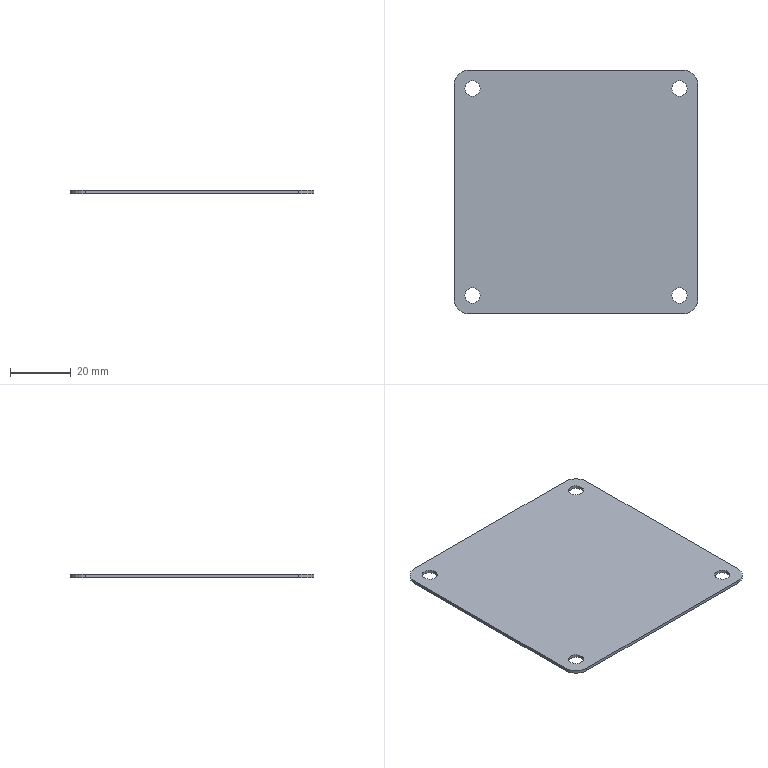Part | SolidWorks | features BaseBody 1 | 1 solid | 18 faces | box 80 x 80 x 1 mm | volume 6300 mm3 | cylinder 12 | plane 6 | commonest cylinder face diameters 5 x8 10 x4
STEP:
#1=CARTESIAN_POINT('',(-36.441,-33.941,1.));
#2=VERTEX_POINT('',#1);
#3=CARTESIAN_POINT('',(-31.441,-33.941,1.));
#4=VERTEX_POINT('',#3);
#5=CARTESIAN_POINT('',(-33.941,-33.941,1.));
#6=DIRECTION('',(0.,0.,1.));
#7=DIRECTION('',(-1.,0.,0.));
#8=AXIS2_PLACEMENT_3D('',#5,#6,#7);
#9=CIRCLE('',#8,2.5);
#10=EDGE_CURVE('',#2,#4,#9,.T.);
#11=ORIENTED_EDGE('',*,*,#10,.T.);
#12=CARTESIAN_POINT('',(-31.441,-33.941,0.));
#13=VERTEX_POINT('',#12);
#14=CARTESIAN_POINT('',(-31.441,-33.941,1.));
#15=DIRECTION('',(0.,0.,-1.));
#16=VECTOR('',#15,1000.);
#17=LINE('',#14,#16);
#18=EDGE_CURVE('',#4,#13,#17,.T.);
#19=ORIENTED_EDGE('',*,*,#18,.T.);
#20=CARTESIAN_POINT('',(-36.441,-33.941,0.));
#21=VERTEX_POINT('',#20);
#22=CARTESIAN_POINT('',(-33.941,-33.941,0.));
#23=DIRECTION('',(0.,0.,1.));
#24=DIRECTION('',(-1.,0.,0.));
#25=AXIS2_PLACEMENT_3D('',#22,#23,#24);
#26=CIRCLE('',#25,2.5);
#27=EDGE_CURVE('',#21,#13,#26,.T.);
#28=ORIENTED_EDGE('',*,*,#27,.F.);
#29=CARTESIAN_POINT('',(-36.441,-33.941,1.));
#30=DIRECTION('',(0.,0.,-1.));
#31=VECTOR('',#30,1000.);
#32=LINE('',#29,#31);
#33=EDGE_CURVE('',#2,#21,#32,.T.);
#34=ORIENTED_EDGE('',*,*,#33,.F.);
#35=EDGE_LOOP('',(#11,#19,#28,#34));
#36=FACE_OUTER_BOUND('',#35,.T.);
#37=CARTESIAN_POINT('',(-33.941,-33.941,1.));
#38=DIRECTION('',(0.,0.,-1.));
#39=DIRECTION('',(-1.,0.,0.));
#40=AXIS2_PLACEMENT_3D('',#37,#38,#39);
#41=CYLINDRICAL_SURFACE('',#40,2.5);
#42=ADVANCED_FACE('',(#36),#41,.F.);
#43=CARTESIAN_POINT('',(31.441,-33.941,1.));
#44=VERTEX_POINT('',#43);
#45=CARTESIAN_POINT('',(36.441,-33.941,1.));
#46=VERTEX_POINT('',#45);
#47=CARTESIAN_POINT('',(33.941,-33.941,1.));
#48=DIRECTION('',(0.,0.,1.));
#49=DIRECTION('',(-1.,0.,0.));
#50=AXIS2_PLACEMENT_3D('',#47,#48,#49);
#51=CIRCLE('',#50,2.5);
#52=EDGE_CURVE('',#44,#46,#51,.T.);
#53=ORIENTED_EDGE('',*,*,#52,.T.);
#54=CARTESIAN_POINT('',(36.441,-33.941,0.));
#55=VERTEX_POINT('',#54);
#56=CARTESIAN_POINT('',(36.441,-33.941,1.));
#57=DIRECTION('',(0.,0.,-1.));
#58=VECTOR('',#57,1000.);
#59=LINE('',#56,#58);
#60=EDGE_CURVE('',#46,#55,#59,.T.);
#61=ORIENTED_EDGE('',*,*,#60,.T.);
#62=CARTESIAN_POINT('',(31.441,-33.941,0.));
#63=VERTEX_POINT('',#62);
#64=CARTESIAN_POINT('',(33.941,-33.941,0.));
#65=DIRECTION('',(0.,0.,1.));
#66=DIRECTION('',(-1.,0.,0.));
#67=AXIS2_PLACEMENT_3D('',#64,#65,#66);
#68=CIRCLE('',#67,2.5);
#69=EDGE_CURVE('',#63,#55,#68,.T.);
#70=ORIENTED_EDGE('',*,*,#69,.F.);
#71=CARTESIAN_POINT('',(31.441,-33.941,1.));
#72=DIRECTION('',(0.,0.,-1.));
#73=VECTOR('',#72,1000.);
#74=LINE('',#71,#73);
#75=EDGE_CURVE('',#44,#63,#74,.T.);
#76=ORIENTED_EDGE('',*,*,#75,.F.);
#77=EDGE_LOOP('',(#53,#61,#70,#76));
#78=FACE_OUTER_BOUND('',#77,.T.);
#79=CARTESIAN_POINT('',(33.941,-33.941,1.));
#80=DIRECTION('',(0.,0.,-1.));
#81=DIRECTION('',(-1.,0.,0.));
#82=AXIS2_PLACEMENT_3D('',#79,#80,#81);
#83=CYLINDRICAL_SURFACE('',#82,2.5);
#84=ADVANCED_FACE('',(#78),#83,.F.);
#85=CARTESIAN_POINT('',(31.441,33.941,1.));
#86=VERTEX_POINT('',#85);
#87=CARTESIAN_POINT('',(36.441,33.941,1.));
#88=VERTEX_POINT('',#87);
#89=CARTESIAN_POINT('',(33.941,33.941,1.));
#90=DIRECTION('',(0.,0.,1.));
#91=DIRECTION('',(-1.,0.,0.));
#92=AXIS2_PLACEMENT_3D('',#89,#90,#91);
#93=CIRCLE('',#92,2.5);
#94=EDGE_CURVE('',#86,#88,#93,.T.);
#95=ORIENTED_EDGE('',*,*,#94,.T.);
#96=CARTESIAN_POINT('',(36.441,33.941,0.));
#97=VERTEX_POINT('',#96);
#98=CARTESIAN_POINT('',(36.441,33.941,1.));
#99=DIRECTION('',(0.,0.,-1.));
#100=VECTOR('',#99,1000.);
#101=LINE('',#98,#100);
#102=EDGE_CURVE('',#88,#97,#101,.T.);
#103=ORIENTED_EDGE('',*,*,#102,.T.);
#104=CARTESIAN_POINT('',(31.441,33.941,0.));
#105=VERTEX_POINT('',#104);
#106=CARTESIAN_POINT('',(33.941,33.941,0.));
#107=DIRECTION('',(0.,0.,1.));
#108=DIRECTION('',(-1.,0.,0.));
#109=AXIS2_PLACEMENT_3D('',#106,#107,#108);
#110=CIRCLE('',#109,2.5);
#111=EDGE_CURVE('',#105,#97,#110,.T.);
#112=ORIENTED_EDGE('',*,*,#111,.F.);
#113=CARTESIAN_POINT('',(31.441,33.941,1.));
#114=DIRECTION('',(0.,0.,-1.));
#115=VECTOR('',#114,1000.);
#116=LINE('',#113,#115);
#117=EDGE_CURVE('',#86,#105,#116,.T.);
#118=ORIENTED_EDGE('',*,*,#117,.F.);
#119=EDGE_LOOP('',(#95,#103,#112,#118));
#120=FACE_OUTER_BOUND('',#119,.T.);
#121=CARTESIAN_POINT('',(33.941,33.941,1.));
#122=DIRECTION('',(0.,0.,-1.));
#123=DIRECTION('',(-1.,0.,0.));
#124=AXIS2_PLACEMENT_3D('',#121,#122,#123);
#125=CYLINDRICAL_SURFACE('',#124,2.5);
#126=ADVANCED_FACE('',(#120),#125,.F.);
#127=CARTESIAN_POINT('',(-36.441,33.941,1.));
#128=VERTEX_POINT('',#127);
#129=CARTESIAN_POINT('',(-31.441,33.941,1.));
#130=VERTEX_POINT('',#129);
#131=CARTESIAN_POINT('',(-33.941,33.941,1.));
#132=DIRECTION('',(0.,0.,1.));
#133=DIRECTION('',(-1.,0.,0.));
#134=AXIS2_PLACEMENT_3D('',#131,#132,#133);
#135=CIRCLE('',#134,2.5);
#136=EDGE_CURVE('',#128,#130,#135,.T.);
#137=ORIENTED_EDGE('',*,*,#136,.T.);
#138=CARTESIAN_POINT('',(-31.441,33.941,0.));
#139=VERTEX_POINT('',#138);
#140=CARTESIAN_POINT('',(-31.441,33.941,1.));
#141=DIRECTION('',(0.,0.,-1.));
#142=VECTOR('',#141,1000.);
#143=LINE('',#140,#142);
#144=EDGE_CURVE('',#130,#139,#143,.T.);
#145=ORIENTED_EDGE('',*,*,#144,.T.);
#146=CARTESIAN_POINT('',(-36.441,33.941,0.));
#147=VERTEX_POINT('',#146);
#148=CARTESIAN_POINT('',(-33.941,33.941,0.));
#149=DIRECTION('',(0.,0.,1.));
#150=DIRECTION('',(-1.,0.,0.));
#151=AXIS2_PLACEMENT_3D('',#148,#149,#150);
#152=CIRCLE('',#151,2.5);
#153=EDGE_CURVE('',#147,#139,#152,.T.);
#154=ORIENTED_EDGE('',*,*,#153,.F.);
#155=CARTESIAN_POINT('',(-36.441,33.941,1.));
#156=DIRECTION('',(0.,0.,-1.));
#157=VECTOR('',#156,1000.);
#158=LINE('',#155,#157);
#159=EDGE_CURVE('',#128,#147,#158,.T.);
#160=ORIENTED_EDGE('',*,*,#159,.F.);
#161=EDGE_LOOP('',(#137,#145,#154,#160));
#162=FACE_OUTER_BOUND('',#161,.T.);
#163=CARTESIAN_POINT('',(-33.941,33.941,1.));
#164=DIRECTION('',(0.,0.,-1.));
#165=DIRECTION('',(-1.,0.,0.));
#166=AXIS2_PLACEMENT_3D('',#163,#164,#165);
#167=CYLINDRICAL_SURFACE('',#166,2.5);
#168=ADVANCED_FACE('',(#162),#167,.F.);
#169=ORIENTED_EDGE('',*,*,#10,.F.);
#170=CARTESIAN_POINT('',(-33.941,-33.941,1.));
#171=DIRECTION('',(0.,0.,1.));
#172=DIRECTION('',(-1.,0.,0.));
#173=AXIS2_PLACEMENT_3D('',#170,#171,#172);
#174=CIRCLE('',#173,2.5);
#175=EDGE_CURVE('',#4,#2,#174,.T.);
#176=ORIENTED_EDGE('',*,*,#175,.F.);
#177=EDGE_LOOP('',(#169,#176));
#178=FACE_BOUND('',#177,.T.);
#179=ORIENTED_EDGE('',*,*,#52,.F.);
#180=CARTESIAN_POINT('',(33.941,-33.941,1.));
#181=DIRECTION('',(0.,0.,1.));
#182=DIRECTION('',(-1.,0.,0.));
#183=AXIS2_PLACEMENT_3D('',#180,#181,#182);
#184=CIRCLE('',#183,2.5);
#185=EDGE_CURVE('',#46,#44,#184,.T.);
#186=ORIENTED_EDGE('',*,*,#185,.F.);
#187=EDGE_LOOP('',(#179,#186));
#188=FACE_BOUND('',#187,.T.);
#189=ORIENTED_EDGE('',*,*,#94,.F.);
#190=CARTESIAN_POINT('',(33.941,33.941,1.));
#191=DIRECTION('',(0.,0.,1.));
#192=DIRECTION('',(-1.,0.,0.));
#193=AXIS2_PLACEMENT_3D('',#190,#191,#192);
#194=CIRCLE('',#193,2.5);
#195=EDGE_CURVE('',#88,#86,#194,.T.);
#196=ORIENTED_EDGE('',*,*,#195,.F.);
#197=EDGE_LOOP('',(#189,#196));
#198=FACE_BOUND('',#197,.T.);
#199=ORIENTED_EDGE('',*,*,#136,.F.);
#200=CARTESIAN_POINT('',(-33.941,33.941,1.));
#201=DIRECTION('',(0.,0.,1.));
#202=DIRECTION('',(-1.,0.,0.));
#203=AXIS2_PLACEMENT_3D('',#200,#201,#202);
#204=CIRCLE('',#203,2.5);
#205=EDGE_CURVE('',#130,#128,#204,.T.);
#206=ORIENTED_EDGE('',*,*,#205,.F.);
#207=EDGE_LOOP('',(#199,#206));
#208=FACE_BOUND('',#207,.T.);
#209=CARTESIAN_POINT('',(35.,-40.,1.));
#210=VERTEX_POINT('',#209);
#211=CARTESIAN_POINT('',(-35.,-40.,1.));
#212=VERTEX_POINT('',#211);
#213=CARTESIAN_POINT('',(-35.,-40.,1.));
#214=DIRECTION('',(-1.,0.,0.));
#215=VECTOR('',#214,1000.);
#216=LINE('',#213,#215);
#217=EDGE_CURVE('',#210,#212,#216,.T.);
#218=ORIENTED_EDGE('',*,*,#217,.F.);
#219=CARTESIAN_POINT('',(40.,-35.,1.));
#220=VERTEX_POINT('',#219);
#221=CARTESIAN_POINT('',(35.,-35.,1.));
#222=DIRECTION('',(0.,0.,-1.));
#223=DIRECTION('',(-1.,0.,0.));
#224=AXIS2_PLACEMENT_3D('',#221,#222,#223);
#225=CIRCLE('',#224,5.);
#226=EDGE_CURVE('',#220,#210,#225,.T.);
#227=ORIENTED_EDGE('',*,*,#226,.F.);
#228=CARTESIAN_POINT('',(40.,35.,1.));
#229=VERTEX_POINT('',#228);
#230=CARTESIAN_POINT('',(40.,-35.,1.));
#231=DIRECTION('',(0.,-1.,0.));
#232=VECTOR('',#231,1000.);
#233=LINE('',#230,#232);
#234=EDGE_CURVE('',#229,#220,#233,.T.);
#235=ORIENTED_EDGE('',*,*,#234,.F.);
#236=CARTESIAN_POINT('',(35.,40.,1.));
#237=VERTEX_POINT('',#236);
#238=CARTESIAN_POINT('',(35.,35.,1.));
#239=DIRECTION('',(0.,0.,-1.));
#240=DIRECTION('',(-1.,0.,0.));
#241=AXIS2_PLACEMENT_3D('',#238,#239,#240);
#242=CIRCLE('',#241,5.);
#243=EDGE_CURVE('',#237,#229,#242,.T.);
#244=ORIENTED_EDGE('',*,*,#243,.F.);
#245=CARTESIAN_POINT('',(-35.,40.,1.));
#246=VERTEX_POINT('',#245);
#247=CARTESIAN_POINT('',(-35.,40.,1.));
#248=DIRECTION('',(1.,0.,0.));
#249=VECTOR('',#248,1000.);
#250=LINE('',#247,#249);
#251=EDGE_CURVE('',#246,#237,#250,.T.);
#252=ORIENTED_EDGE('',*,*,#251,.F.);
#253=CARTESIAN_POINT('',(-40.,35.,1.));
#254=VERTEX_POINT('',#253);
#255=CARTESIAN_POINT('',(-35.,35.,1.));
#256=DIRECTION('',(0.,0.,-1.));
#257=DIRECTION('',(-1.,0.,0.));
#258=AXIS2_PLACEMENT_3D('',#255,#256,#257);
#259=CIRCLE('',#258,5.);
#260=EDGE_CURVE('',#254,#246,#259,.T.);
#261=ORIENTED_EDGE('',*,*,#260,.F.);
#262=CARTESIAN_POINT('',(-40.,-35.,1.));
#263=VERTEX_POINT('',#262);
#264=CARTESIAN_POINT('',(-40.,-35.,1.));
#265=DIRECTION('',(0.,1.,0.));
#266=VECTOR('',#265,1000.);
#267=LINE('',#264,#266);
#268=EDGE_CURVE('',#263,#254,#267,.T.);
#269=ORIENTED_EDGE('',*,*,#268,.F.);
#270=CARTESIAN_POINT('',(-35.,-35.,1.));
#271=DIRECTION('',(0.,0.,-1.));
#272=DIRECTION('',(-1.,0.,0.));
#273=AXIS2_PLACEMENT_3D('',#270,#271,#272);
#274=CIRCLE('',#273,5.);
#275=EDGE_CURVE('',#212,#263,#274,.T.);
#276=ORIENTED_EDGE('',*,*,#275,.F.);
#277=EDGE_LOOP('',(#218,#227,#235,#244,#252,#261,#269,#276));
#278=FACE_OUTER_BOUND('',#277,.T.);
#279=CARTESIAN_POINT('',(-35.,-35.,1.));
#280=DIRECTION('',(0.,0.,-1.));
#281=DIRECTION('',(-1.,0.,0.));
#282=AXIS2_PLACEMENT_3D('',#279,#280,#281);
#283=PLANE('',#282);
#284=ADVANCED_FACE('',(#178,#188,#198,#208,#278),#283,.F.);
#285=ORIENTED_EDGE('',*,*,#18,.F.);
#286=ORIENTED_EDGE('',*,*,#175,.T.);
#287=ORIENTED_EDGE('',*,*,#33,.T.);
#288=CARTESIAN_POINT('',(-33.941,-33.941,0.));
#289=DIRECTION('',(0.,0.,1.));
#290=DIRECTION('',(-1.,0.,0.));
#291=AXIS2_PLACEMENT_3D('',#288,#289,#290);
#292=CIRCLE('',#291,2.5);
#293=EDGE_CURVE('',#13,#21,#292,.T.);
#294=ORIENTED_EDGE('',*,*,#293,.F.);
#295=EDGE_LOOP('',(#285,#286,#287,#294));
#296=FACE_OUTER_BOUND('',#295,.T.);
#297=CARTESIAN_POINT('',(-33.941,-33.941,1.));
#298=DIRECTION('',(0.,0.,-1.));
#299=DIRECTION('',(-1.,0.,0.));
#300=AXIS2_PLACEMENT_3D('',#297,#298,#299);
#301=CYLINDRICAL_SURFACE('',#300,2.5);
#302=ADVANCED_FACE('',(#296),#301,.F.);
#303=ORIENTED_EDGE('',*,*,#60,.F.);
#304=ORIENTED_EDGE('',*,*,#185,.T.);
#305=ORIENTED_EDGE('',*,*,#75,.T.);
#306=CARTESIAN_POINT('',(33.941,-33.941,0.));
#307=DIRECTION('',(0.,0.,1.));
#308=DIRECTION('',(-1.,0.,0.));
#309=AXIS2_PLACEMENT_3D('',#306,#307,#308);
#310=CIRCLE('',#309,2.5);
#311=EDGE_CURVE('',#55,#63,#310,.T.);
#312=ORIENTED_EDGE('',*,*,#311,.F.);
#313=EDGE_LOOP('',(#303,#304,#305,#312));
#314=FACE_OUTER_BOUND('',#313,.T.);
#315=CARTESIAN_POINT('',(33.941,-33.941,1.));
#316=DIRECTION('',(0.,0.,-1.));
#317=DIRECTION('',(-1.,0.,0.));
#318=AXIS2_PLACEMENT_3D('',#315,#316,#317);
#319=CYLINDRICAL_SURFACE('',#318,2.5);
#320=ADVANCED_FACE('',(#314),#319,.F.);
#321=ORIENTED_EDGE('',*,*,#102,.F.);
#322=ORIENTED_EDGE('',*,*,#195,.T.);
#323=ORIENTED_EDGE('',*,*,#117,.T.);
#324=CARTESIAN_POINT('',(33.941,33.941,0.));
#325=DIRECTION('',(0.,0.,1.));
#326=DIRECTION('',(-1.,0.,0.));
#327=AXIS2_PLACEMENT_3D('',#324,#325,#326);
#328=CIRCLE('',#327,2.5);
#329=EDGE_CURVE('',#97,#105,#328,.T.);
#330=ORIENTED_EDGE('',*,*,#329,.F.);
#331=EDGE_LOOP('',(#321,#322,#323,#330));
#332=FACE_OUTER_BOUND('',#331,.T.);
#333=CARTESIAN_POINT('',(33.941,33.941,1.));
#334=DIRECTION('',(0.,0.,-1.));
#335=DIRECTION('',(-1.,0.,0.));
#336=AXIS2_PLACEMENT_3D('',#333,#334,#335);
#337=CYLINDRICAL_SURFACE('',#336,2.5);
#338=ADVANCED_FACE('',(#332),#337,.F.);
#339=ORIENTED_EDGE('',*,*,#144,.F.);
#340=ORIENTED_EDGE('',*,*,#205,.T.);
#341=ORIENTED_EDGE('',*,*,#159,.T.);
#342=CARTESIAN_POINT('',(-33.941,33.941,0.));
#343=DIRECTION('',(0.,0.,1.));
#344=DIRECTION('',(-1.,0.,0.));
#345=AXIS2_PLACEMENT_3D('',#342,#343,#344);
#346=CIRCLE('',#345,2.5);
#347=EDGE_CURVE('',#139,#147,#346,.T.);
#348=ORIENTED_EDGE('',*,*,#347,.F.);
#349=EDGE_LOOP('',(#339,#340,#341,#348));
#350=FACE_OUTER_BOUND('',#349,.T.);
#351=CARTESIAN_POINT('',(-33.941,33.941,1.));
#352=DIRECTION('',(0.,0.,-1.));
#353=DIRECTION('',(-1.,0.,0.));
#354=AXIS2_PLACEMENT_3D('',#351,#352,#353);
#355=CYLINDRICAL_SURFACE('',#354,2.5);
#356=ADVANCED_FACE('',(#350),#355,.F.);
#357=ORIENTED_EDGE('',*,*,#275,.T.);
#358=CARTESIAN_POINT('',(-40.,-35.,0.));
#359=VERTEX_POINT('',#358);
#360=CARTESIAN_POINT('',(-40.,-35.,1.));
#361=DIRECTION('',(0.,0.,-1.));
#362=VECTOR('',#361,1000.);
#363=LINE('',#360,#362);
#364=EDGE_CURVE('',#263,#359,#363,.T.);
#365=ORIENTED_EDGE('',*,*,#364,.T.);
#366=CARTESIAN_POINT('',(-35.,-40.,0.));
#367=VERTEX_POINT('',#366);
#368=CARTESIAN_POINT('',(-35.,-35.,0.));
#369=DIRECTION('',(0.,0.,1.));
#370=DIRECTION('',(-1.,0.,0.));
#371=AXIS2_PLACEMENT_3D('',#368,#369,#370);
#372=CIRCLE('',#371,5.);
#373=EDGE_CURVE('',#359,#367,#372,.T.);
#374=ORIENTED_EDGE('',*,*,#373,.T.);
#375=CARTESIAN_POINT('',(-35.,-40.,1.));
#376=DIRECTION('',(0.,0.,1.));
#377=VECTOR('',#376,1000.);
#378=LINE('',#375,#377);
#379=EDGE_CURVE('',#367,#212,#378,.T.);
#380=ORIENTED_EDGE('',*,*,#379,.T.);
#381=EDGE_LOOP('',(#357,#365,#374,#380));
#382=FACE_OUTER_BOUND('',#381,.T.);
#383=CARTESIAN_POINT('',(-35.,-35.,1.));
#384=DIRECTION('',(0.,0.,-1.));
#385=DIRECTION('',(-1.,0.,0.));
#386=AXIS2_PLACEMENT_3D('',#383,#384,#385);
#387=CYLINDRICAL_SURFACE('',#386,5.);
#388=ADVANCED_FACE('',(#382),#387,.T.);
#389=CARTESIAN_POINT('',(35.,-40.,0.));
#390=VERTEX_POINT('',#389);
#391=CARTESIAN_POINT('',(35.,-40.,1.));
#392=DIRECTION('',(0.,0.,-1.));
#393=VECTOR('',#392,1000.);
#394=LINE('',#391,#393);
#395=EDGE_CURVE('',#210,#390,#394,.T.);
#396=ORIENTED_EDGE('',*,*,#395,.F.);
#397=ORIENTED_EDGE('',*,*,#217,.T.);
#398=ORIENTED_EDGE('',*,*,#379,.F.);
#399=CARTESIAN_POINT('',(35.,-40.,0.));
#400=DIRECTION('',(-1.,0.,0.));
#401=VECTOR('',#400,1000.);
#402=LINE('',#399,#401);
#403=EDGE_CURVE('',#390,#367,#402,.T.);
#404=ORIENTED_EDGE('',*,*,#403,.F.);
#405=EDGE_LOOP('',(#396,#397,#398,#404));
#406=FACE_OUTER_BOUND('',#405,.T.);
#407=CARTESIAN_POINT('',(35.,-40.,1.));
#408=DIRECTION('',(0.,1.,0.));
#409=DIRECTION('',(-1.,0.,0.));
#410=AXIS2_PLACEMENT_3D('',#407,#408,#409);
#411=PLANE('',#410);
#412=ADVANCED_FACE('',(#406),#411,.F.);
#413=ORIENTED_EDGE('',*,*,#226,.T.);
#414=ORIENTED_EDGE('',*,*,#395,.T.);
#415=CARTESIAN_POINT('',(40.,-35.,0.));
#416=VERTEX_POINT('',#415);
#417=CARTESIAN_POINT('',(35.,-35.,0.));
#418=DIRECTION('',(0.,0.,1.));
#419=DIRECTION('',(-1.,0.,0.));
#420=AXIS2_PLACEMENT_3D('',#417,#418,#419);
#421=CIRCLE('',#420,5.);
#422=EDGE_CURVE('',#390,#416,#421,.T.);
#423=ORIENTED_EDGE('',*,*,#422,.T.);
#424=CARTESIAN_POINT('',(40.,-35.,1.));
#425=DIRECTION('',(0.,0.,1.));
#426=VECTOR('',#425,1000.);
#427=LINE('',#424,#426);
#428=EDGE_CURVE('',#416,#220,#427,.T.);
#429=ORIENTED_EDGE('',*,*,#428,.T.);
#430=EDGE_LOOP('',(#413,#414,#423,#429));
#431=FACE_OUTER_BOUND('',#430,.T.);
#432=CARTESIAN_POINT('',(35.,-35.,1.));
#433=DIRECTION('',(0.,0.,-1.));
#434=DIRECTION('',(-1.,0.,0.));
#435=AXIS2_PLACEMENT_3D('',#432,#433,#434);
#436=CYLINDRICAL_SURFACE('',#435,5.);
#437=ADVANCED_FACE('',(#431),#436,.T.);
#438=CARTESIAN_POINT('',(40.,35.,0.));
#439=VERTEX_POINT('',#438);
#440=CARTESIAN_POINT('',(40.,35.,1.));
#441=DIRECTION('',(0.,0.,-1.));
#442=VECTOR('',#441,1000.);
#443=LINE('',#440,#442);
#444=EDGE_CURVE('',#229,#439,#443,.T.);
#445=ORIENTED_EDGE('',*,*,#444,.F.);
#446=ORIENTED_EDGE('',*,*,#234,.T.);
#447=ORIENTED_EDGE('',*,*,#428,.F.);
#448=CARTESIAN_POINT('',(40.,35.,0.));
#449=DIRECTION('',(0.,-1.,0.));
#450=VECTOR('',#449,1000.);
#451=LINE('',#448,#450);
#452=EDGE_CURVE('',#439,#416,#451,.T.);
#453=ORIENTED_EDGE('',*,*,#452,.F.);
#454=EDGE_LOOP('',(#445,#446,#447,#453));
#455=FACE_OUTER_BOUND('',#454,.T.);
#456=CARTESIAN_POINT('',(40.,35.,1.));
#457=DIRECTION('',(-1.,0.,0.));
#458=DIRECTION('',(0.,-1.,0.));
#459=AXIS2_PLACEMENT_3D('',#456,#457,#458);
#460=PLANE('',#459);
#461=ADVANCED_FACE('',(#455),#460,.F.);
#462=ORIENTED_EDGE('',*,*,#243,.T.);
#463=ORIENTED_EDGE('',*,*,#444,.T.);
#464=CARTESIAN_POINT('',(35.,40.,0.));
#465=VERTEX_POINT('',#464);
#466=CARTESIAN_POINT('',(35.,35.,0.));
#467=DIRECTION('',(0.,0.,1.));
#468=DIRECTION('',(-1.,0.,0.));
#469=AXIS2_PLACEMENT_3D('',#466,#467,#468);
#470=CIRCLE('',#469,5.);
#471=EDGE_CURVE('',#439,#465,#470,.T.);
#472=ORIENTED_EDGE('',*,*,#471,.T.);
#473=CARTESIAN_POINT('',(35.,40.,1.));
#474=DIRECTION('',(0.,0.,1.));
#475=VECTOR('',#474,1000.);
#476=LINE('',#473,#475);
#477=EDGE_CURVE('',#465,#237,#476,.T.);
#478=ORIENTED_EDGE('',*,*,#477,.T.);
#479=EDGE_LOOP('',(#462,#463,#472,#478));
#480=FACE_OUTER_BOUND('',#479,.T.);
#481=CARTESIAN_POINT('',(35.,35.,1.));
#482=DIRECTION('',(0.,0.,-1.));
#483=DIRECTION('',(-1.,0.,0.));
#484=AXIS2_PLACEMENT_3D('',#481,#482,#483);
#485=CYLINDRICAL_SURFACE('',#484,5.);
#486=ADVANCED_FACE('',(#480),#485,.T.);
#487=CARTESIAN_POINT('',(-35.,40.,0.));
#488=VERTEX_POINT('',#487);
#489=CARTESIAN_POINT('',(-35.,40.,1.));
#490=DIRECTION('',(0.,0.,-1.));
#491=VECTOR('',#490,1000.);
#492=LINE('',#489,#491);
#493=EDGE_CURVE('',#246,#488,#492,.T.);
#494=ORIENTED_EDGE('',*,*,#493,.F.);
#495=ORIENTED_EDGE('',*,*,#251,.T.);
#496=ORIENTED_EDGE('',*,*,#477,.F.);
#497=CARTESIAN_POINT('',(35.,40.,0.));
#498=DIRECTION('',(1.,0.,0.));
#499=VECTOR('',#498,1000.);
#500=LINE('',#497,#499);
#501=EDGE_CURVE('',#488,#465,#500,.T.);
#502=ORIENTED_EDGE('',*,*,#501,.F.);
#503=EDGE_LOOP('',(#494,#495,#496,#502));
#504=FACE_OUTER_BOUND('',#503,.T.);
#505=CARTESIAN_POINT('',(35.,40.,1.));
#506=DIRECTION('',(0.,-1.,0.));
#507=DIRECTION('',(1.,0.,0.));
#508=AXIS2_PLACEMENT_3D('',#505,#506,#507);
#509=PLANE('',#508);
#510=ADVANCED_FACE('',(#504),#509,.F.);
#511=ORIENTED_EDGE('',*,*,#260,.T.);
#512=ORIENTED_EDGE('',*,*,#493,.T.);
#513=CARTESIAN_POINT('',(-40.,35.,0.));
#514=VERTEX_POINT('',#513);
#515=CARTESIAN_POINT('',(-35.,35.,0.));
#516=DIRECTION('',(0.,0.,1.));
#517=DIRECTION('',(-1.,0.,0.));
#518=AXIS2_PLACEMENT_3D('',#515,#516,#517);
#519=CIRCLE('',#518,5.);
#520=EDGE_CURVE('',#488,#514,#519,.T.);
#521=ORIENTED_EDGE('',*,*,#520,.T.);
#522=CARTESIAN_POINT('',(-40.,35.,1.));
#523=DIRECTION('',(0.,0.,1.));
#524=VECTOR('',#523,1000.);
#525=LINE('',#522,#524);
#526=EDGE_CURVE('',#514,#254,#525,.T.);
#527=ORIENTED_EDGE('',*,*,#526,.T.);
#528=EDGE_LOOP('',(#511,#512,#521,#527));
#529=FACE_OUTER_BOUND('',#528,.T.);
#530=CARTESIAN_POINT('',(-35.,35.,1.));
#531=DIRECTION('',(0.,0.,-1.));
#532=DIRECTION('',(-1.,0.,0.));
#533=AXIS2_PLACEMENT_3D('',#530,#531,#532);
#534=CYLINDRICAL_SURFACE('',#533,5.);
#535=ADVANCED_FACE('',(#529),#534,.T.);
#536=ORIENTED_EDGE('',*,*,#364,.F.);
#537=ORIENTED_EDGE('',*,*,#268,.T.);
#538=ORIENTED_EDGE('',*,*,#526,.F.);
#539=CARTESIAN_POINT('',(-40.,35.,0.));
#540=DIRECTION('',(0.,1.,0.));
#541=VECTOR('',#540,1000.);
#542=LINE('',#539,#541);
#543=EDGE_CURVE('',#359,#514,#542,.T.);
#544=ORIENTED_EDGE('',*,*,#543,.F.);
#545=EDGE_LOOP('',(#536,#537,#538,#544));
#546=FACE_OUTER_BOUND('',#545,.T.);
#547=CARTESIAN_POINT('',(-40.,35.,1.));
#548=DIRECTION('',(1.,0.,0.));
#549=DIRECTION('',(0.,0.,-1.));
#550=AXIS2_PLACEMENT_3D('',#547,#548,#549);
#551=PLANE('',#550);
#552=ADVANCED_FACE('',(#546),#551,.F.);
#553=ORIENTED_EDGE('',*,*,#27,.T.);
#554=ORIENTED_EDGE('',*,*,#293,.T.);
#555=EDGE_LOOP('',(#553,#554));
#556=FACE_BOUND('',#555,.T.);
#557=ORIENTED_EDGE('',*,*,#111,.T.);
#558=ORIENTED_EDGE('',*,*,#329,.T.);
#559=EDGE_LOOP('',(#557,#558));
#560=FACE_BOUND('',#559,.T.);
#561=ORIENTED_EDGE('',*,*,#153,.T.);
#562=ORIENTED_EDGE('',*,*,#347,.T.);
#563=EDGE_LOOP('',(#561,#562));
#564=FACE_BOUND('',#563,.T.);
#565=ORIENTED_EDGE('',*,*,#69,.T.);
#566=ORIENTED_EDGE('',*,*,#311,.T.);
#567=EDGE_LOOP('',(#565,#566));
#568=FACE_BOUND('',#567,.T.);
#569=ORIENTED_EDGE('',*,*,#422,.F.);
#570=ORIENTED_EDGE('',*,*,#403,.T.);
#571=ORIENTED_EDGE('',*,*,#373,.F.);
#572=ORIENTED_EDGE('',*,*,#543,.T.);
#573=ORIENTED_EDGE('',*,*,#520,.F.);
#574=ORIENTED_EDGE('',*,*,#501,.T.);
#575=ORIENTED_EDGE('',*,*,#471,.F.);
#576=ORIENTED_EDGE('',*,*,#452,.T.);
#577=EDGE_LOOP('',(#569,#570,#571,#572,#573,#574,#575,#576));
#578=FACE_OUTER_BOUND('',#577,.T.);
#579=CARTESIAN_POINT('',(-35.,-35.,0.));
#580=DIRECTION('',(0.,0.,-1.));
#581=DIRECTION('',(-1.,0.,0.));
#582=AXIS2_PLACEMENT_3D('',#579,#580,#581);
#583=PLANE('',#582);
#584=ADVANCED_FACE('',(#556,#560,#564,#568,#578),#583,.T.);
#585=CLOSED_SHELL('',(#42,#84,#126,#168,#284,#302,#320,#338,#356,#388,#412,#437,#461,#486,#510,#535,#552,#584));
#586=MANIFOLD_SOLID_BREP('',#585);
#587=CARTESIAN_POINT('',(0.,0.,0.));
#588=DIRECTION('',(0.,0.,1.));
#589=DIRECTION('',(1.,0.,0.));
#590=AXIS2_PLACEMENT_3D('',#587,#588,#589);
#591=(LENGTH_UNIT()NAMED_UNIT(*)SI_UNIT(.MILLI.,.METRE.));
#592=UNCERTAINTY_MEASURE_WITH_UNIT(LENGTH_MEASURE(0.00001),#591,'','');
#593=(NAMED_UNIT(*)PLANE_ANGLE_UNIT()SI_UNIT($,.RADIAN.));
#594=(NAMED_UNIT(*)SI_UNIT($,.STERADIAN.)SOLID_ANGLE_UNIT());
#595=(GEOMETRIC_REPRESENTATION_CONTEXT(3)GLOBAL_UNCERTAINTY_ASSIGNED_CONTEXT((#592))GLOBAL_UNIT_ASSIGNED_CONTEXT((#591,#593,#594))REPRESENTATION_CONTEXT('',''));
#596=ADVANCED_BREP_SHAPE_REPRESENTATION('',(#586,#590),#595);